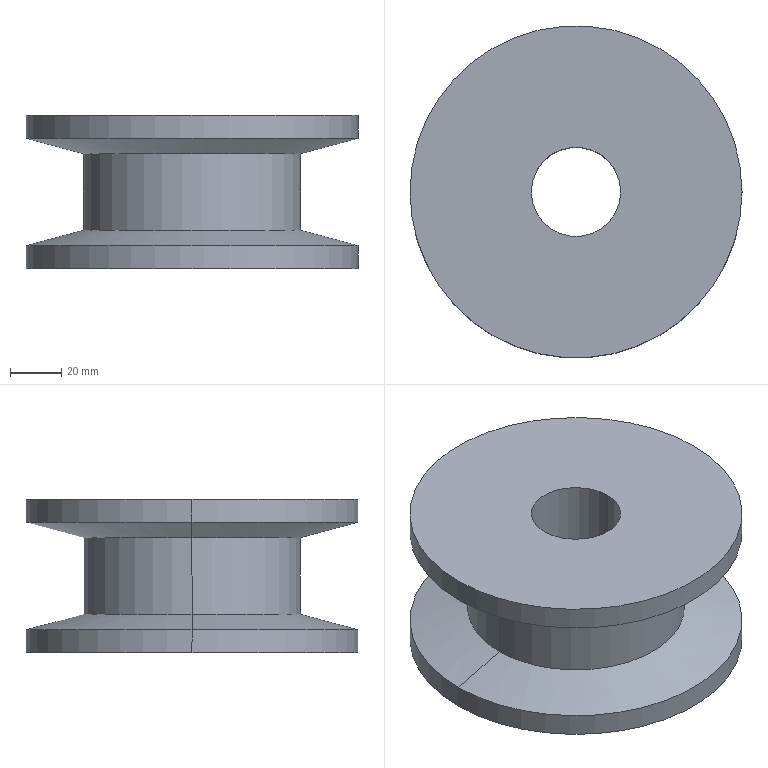Part | SolidWorks | features BaseBody 1 | 1 solid | 14 faces | box 130 x 130 x 60 mm | volume 461932 mm3 | cylinder 8 | cone 4 | plane 2 | commonest cylinder face diameters 130 x4 35 x2 85 x2
STEP:
#1=CARTESIAN_POINT('',(65.,0.,21.));
#2=VERTEX_POINT('',#1);
#3=CARTESIAN_POINT('',(-65.,0.,21.));
#4=VERTEX_POINT('',#3);
#5=CARTESIAN_POINT('',(0.,0.,21.));
#6=DIRECTION('',(0.,0.,1.));
#7=DIRECTION('',(1.,0.,0.));
#8=AXIS2_PLACEMENT_3D('',#5,#6,#7);
#9=CIRCLE('',#8,65.);
#10=EDGE_CURVE('',#2,#4,#9,.T.);
#11=ORIENTED_EDGE('',*,*,#10,.T.);
#12=CARTESIAN_POINT('',(-65.,0.,30.));
#13=VERTEX_POINT('',#12);
#14=CARTESIAN_POINT('',(-65.,0.,0.));
#15=DIRECTION('',(0.,0.,1.));
#16=VECTOR('',#15,1000.);
#17=LINE('',#14,#16);
#18=EDGE_CURVE('',#4,#13,#17,.T.);
#19=ORIENTED_EDGE('',*,*,#18,.T.);
#20=CARTESIAN_POINT('',(65.,0.,30.));
#21=VERTEX_POINT('',#20);
#22=CARTESIAN_POINT('',(0.,0.,30.));
#23=DIRECTION('',(0.,0.,-1.));
#24=DIRECTION('',(1.,0.,0.));
#25=AXIS2_PLACEMENT_3D('',#22,#23,#24);
#26=CIRCLE('',#25,65.);
#27=EDGE_CURVE('',#13,#21,#26,.T.);
#28=ORIENTED_EDGE('',*,*,#27,.T.);
#29=CARTESIAN_POINT('',(65.,0.,0.));
#30=DIRECTION('',(0.,0.,1.));
#31=VECTOR('',#30,1000.);
#32=LINE('',#29,#31);
#33=EDGE_CURVE('',#2,#21,#32,.T.);
#34=ORIENTED_EDGE('',*,*,#33,.F.);
#35=EDGE_LOOP('',(#11,#19,#28,#34));
#36=FACE_OUTER_BOUND('',#35,.T.);
#37=CARTESIAN_POINT('',(0.,0.,0.));
#38=DIRECTION('',(0.,0.,1.));
#39=DIRECTION('',(1.,0.,0.));
#40=AXIS2_PLACEMENT_3D('',#37,#38,#39);
#41=CYLINDRICAL_SURFACE('',#40,65.);
#42=ADVANCED_FACE('',(#36),#41,.T.);
#43=CARTESIAN_POINT('',(-17.5,0.,-30.));
#44=VERTEX_POINT('',#43);
#45=CARTESIAN_POINT('',(17.5,0.,-30.));
#46=VERTEX_POINT('',#45);
#47=CARTESIAN_POINT('',(0.,0.,-30.));
#48=DIRECTION('',(0.,0.,1.));
#49=DIRECTION('',(1.,0.,0.));
#50=AXIS2_PLACEMENT_3D('',#47,#48,#49);
#51=CIRCLE('',#50,17.5);
#52=EDGE_CURVE('',#44,#46,#51,.T.);
#53=ORIENTED_EDGE('',*,*,#52,.F.);
#54=CARTESIAN_POINT('',(-17.5,0.,30.));
#55=VERTEX_POINT('',#54);
#56=CARTESIAN_POINT('',(-17.5,0.,0.));
#57=DIRECTION('',(0.,0.,1.));
#58=VECTOR('',#57,1000.);
#59=LINE('',#56,#58);
#60=EDGE_CURVE('',#44,#55,#59,.T.);
#61=ORIENTED_EDGE('',*,*,#60,.T.);
#62=CARTESIAN_POINT('',(17.5,0.,30.));
#63=VERTEX_POINT('',#62);
#64=CARTESIAN_POINT('',(0.,0.,30.));
#65=DIRECTION('',(0.,0.,1.));
#66=DIRECTION('',(1.,0.,0.));
#67=AXIS2_PLACEMENT_3D('',#64,#65,#66);
#68=CIRCLE('',#67,17.5);
#69=EDGE_CURVE('',#55,#63,#68,.T.);
#70=ORIENTED_EDGE('',*,*,#69,.T.);
#71=CARTESIAN_POINT('',(17.5,0.,0.));
#72=DIRECTION('',(0.,0.,1.));
#73=VECTOR('',#72,1000.);
#74=LINE('',#71,#73);
#75=EDGE_CURVE('',#46,#63,#74,.T.);
#76=ORIENTED_EDGE('',*,*,#75,.F.);
#77=EDGE_LOOP('',(#53,#61,#70,#76));
#78=FACE_OUTER_BOUND('',#77,.T.);
#79=CARTESIAN_POINT('',(0.,0.,0.));
#80=DIRECTION('',(0.,0.,1.));
#81=DIRECTION('',(1.,0.,0.));
#82=AXIS2_PLACEMENT_3D('',#79,#80,#81);
#83=CYLINDRICAL_SURFACE('',#82,17.5);
#84=ADVANCED_FACE('',(#78),#83,.F.);
#85=CARTESIAN_POINT('',(42.5,0.,15.));
#86=VERTEX_POINT('',#85);
#87=CARTESIAN_POINT('',(-42.5,0.,15.));
#88=VERTEX_POINT('',#87);
#89=CARTESIAN_POINT('',(0.,0.,15.));
#90=DIRECTION('',(0.,0.,1.));
#91=DIRECTION('',(1.,0.,0.));
#92=AXIS2_PLACEMENT_3D('',#89,#90,#91);
#93=CIRCLE('',#92,42.5);
#94=EDGE_CURVE('',#86,#88,#93,.T.);
#95=ORIENTED_EDGE('',*,*,#94,.T.);
#96=CARTESIAN_POINT('',(-65.,0.,21.));
#97=DIRECTION('',(-0.9662,0.,0.2577));
#98=VECTOR('',#97,1000.);
#99=LINE('',#96,#98);
#100=EDGE_CURVE('',#88,#4,#99,.T.);
#101=ORIENTED_EDGE('',*,*,#100,.T.);
#102=ORIENTED_EDGE('',*,*,#10,.F.);
#103=CARTESIAN_POINT('',(65.,0.,21.));
#104=DIRECTION('',(0.9662,0.,0.2577));
#105=VECTOR('',#104,1000.);
#106=LINE('',#103,#105);
#107=EDGE_CURVE('',#86,#2,#106,.T.);
#108=ORIENTED_EDGE('',*,*,#107,.F.);
#109=EDGE_LOOP('',(#95,#101,#102,#108));
#110=FACE_OUTER_BOUND('',#109,.T.);
#111=CARTESIAN_POINT('',(0.,0.,21.));
#112=DIRECTION('',(0.,0.,1.));
#113=DIRECTION('',(1.,0.,0.));
#114=AXIS2_PLACEMENT_3D('',#111,#112,#113);
#115=CONICAL_SURFACE('',#114,65.,1.31);
#116=ADVANCED_FACE('',(#110),#115,.T.);
#117=CARTESIAN_POINT('',(42.5,0.,-15.));
#118=VERTEX_POINT('',#117);
#119=CARTESIAN_POINT('',(-42.5,0.,-15.));
#120=VERTEX_POINT('',#119);
#121=CARTESIAN_POINT('',(0.,0.,-15.));
#122=DIRECTION('',(0.,0.,1.));
#123=DIRECTION('',(1.,0.,0.));
#124=AXIS2_PLACEMENT_3D('',#121,#122,#123);
#125=CIRCLE('',#124,42.5);
#126=EDGE_CURVE('',#118,#120,#125,.T.);
#127=ORIENTED_EDGE('',*,*,#126,.T.);
#128=CARTESIAN_POINT('',(-42.5,0.,0.));
#129=DIRECTION('',(0.,0.,1.));
#130=VECTOR('',#129,1000.);
#131=LINE('',#128,#130);
#132=EDGE_CURVE('',#120,#88,#131,.T.);
#133=ORIENTED_EDGE('',*,*,#132,.T.);
#134=ORIENTED_EDGE('',*,*,#94,.F.);
#135=CARTESIAN_POINT('',(42.5,0.,0.));
#136=DIRECTION('',(0.,0.,1.));
#137=VECTOR('',#136,1000.);
#138=LINE('',#135,#137);
#139=EDGE_CURVE('',#118,#86,#138,.T.);
#140=ORIENTED_EDGE('',*,*,#139,.F.);
#141=EDGE_LOOP('',(#127,#133,#134,#140));
#142=FACE_OUTER_BOUND('',#141,.T.);
#143=CARTESIAN_POINT('',(0.,0.,0.));
#144=DIRECTION('',(0.,0.,1.));
#145=DIRECTION('',(1.,0.,0.));
#146=AXIS2_PLACEMENT_3D('',#143,#144,#145);
#147=CYLINDRICAL_SURFACE('',#146,42.5);
#148=ADVANCED_FACE('',(#142),#147,.T.);
#149=CARTESIAN_POINT('',(65.,0.,-30.));
#150=VERTEX_POINT('',#149);
#151=CARTESIAN_POINT('',(-65.,0.,-30.));
#152=VERTEX_POINT('',#151);
#153=CARTESIAN_POINT('',(0.,0.,-30.));
#154=DIRECTION('',(0.,0.,1.));
#155=DIRECTION('',(1.,0.,0.));
#156=AXIS2_PLACEMENT_3D('',#153,#154,#155);
#157=CIRCLE('',#156,65.);
#158=EDGE_CURVE('',#150,#152,#157,.T.);
#159=ORIENTED_EDGE('',*,*,#158,.T.);
#160=CARTESIAN_POINT('',(-65.,0.,-21.));
#161=VERTEX_POINT('',#160);
#162=CARTESIAN_POINT('',(-65.,0.,0.));
#163=DIRECTION('',(0.,0.,1.));
#164=VECTOR('',#163,1000.);
#165=LINE('',#162,#164);
#166=EDGE_CURVE('',#152,#161,#165,.T.);
#167=ORIENTED_EDGE('',*,*,#166,.T.);
#168=CARTESIAN_POINT('',(65.,0.,-21.));
#169=VERTEX_POINT('',#168);
#170=CARTESIAN_POINT('',(0.,0.,-21.));
#171=DIRECTION('',(0.,0.,-1.));
#172=DIRECTION('',(1.,0.,0.));
#173=AXIS2_PLACEMENT_3D('',#170,#171,#172);
#174=CIRCLE('',#173,65.);
#175=EDGE_CURVE('',#161,#169,#174,.T.);
#176=ORIENTED_EDGE('',*,*,#175,.T.);
#177=CARTESIAN_POINT('',(65.,0.,0.));
#178=DIRECTION('',(0.,0.,1.));
#179=VECTOR('',#178,1000.);
#180=LINE('',#177,#179);
#181=EDGE_CURVE('',#150,#169,#180,.T.);
#182=ORIENTED_EDGE('',*,*,#181,.F.);
#183=EDGE_LOOP('',(#159,#167,#176,#182));
#184=FACE_OUTER_BOUND('',#183,.T.);
#185=CARTESIAN_POINT('',(0.,0.,0.));
#186=DIRECTION('',(0.,0.,1.));
#187=DIRECTION('',(1.,0.,0.));
#188=AXIS2_PLACEMENT_3D('',#185,#186,#187);
#189=CYLINDRICAL_SURFACE('',#188,65.);
#190=ADVANCED_FACE('',(#184),#189,.T.);
#191=ORIENTED_EDGE('',*,*,#126,.F.);
#192=CARTESIAN_POINT('',(65.,0.,-21.));
#193=DIRECTION('',(0.9662,0.,-0.2577));
#194=VECTOR('',#193,1000.);
#195=LINE('',#192,#194);
#196=EDGE_CURVE('',#118,#169,#195,.T.);
#197=ORIENTED_EDGE('',*,*,#196,.T.);
#198=ORIENTED_EDGE('',*,*,#175,.F.);
#199=CARTESIAN_POINT('',(-65.,0.,-21.));
#200=DIRECTION('',(-0.9662,0.,-0.2577));
#201=VECTOR('',#200,1000.);
#202=LINE('',#199,#201);
#203=EDGE_CURVE('',#120,#161,#202,.T.);
#204=ORIENTED_EDGE('',*,*,#203,.F.);
#205=EDGE_LOOP('',(#191,#197,#198,#204));
#206=FACE_OUTER_BOUND('',#205,.T.);
#207=CARTESIAN_POINT('',(0.,0.,-21.));
#208=DIRECTION('',(0.,0.,-1.));
#209=DIRECTION('',(-1.,0.,0.));
#210=AXIS2_PLACEMENT_3D('',#207,#208,#209);
#211=CONICAL_SURFACE('',#210,65.,1.31);
#212=ADVANCED_FACE('',(#206),#211,.T.);
#213=CARTESIAN_POINT('',(0.,0.,30.));
#214=DIRECTION('',(0.,0.,-1.));
#215=DIRECTION('',(1.,0.,0.));
#216=AXIS2_PLACEMENT_3D('',#213,#214,#215);
#217=CIRCLE('',#216,65.);
#218=EDGE_CURVE('',#21,#13,#217,.T.);
#219=ORIENTED_EDGE('',*,*,#218,.F.);
#220=ORIENTED_EDGE('',*,*,#27,.F.);
#221=EDGE_LOOP('',(#219,#220));
#222=FACE_OUTER_BOUND('',#221,.T.);
#223=CARTESIAN_POINT('',(0.,0.,30.));
#224=DIRECTION('',(0.,0.,1.));
#225=DIRECTION('',(1.,0.,0.));
#226=AXIS2_PLACEMENT_3D('',#223,#224,#225);
#227=CIRCLE('',#226,17.5);
#228=EDGE_CURVE('',#63,#55,#227,.T.);
#229=ORIENTED_EDGE('',*,*,#228,.F.);
#230=ORIENTED_EDGE('',*,*,#69,.F.);
#231=EDGE_LOOP('',(#229,#230));
#232=FACE_BOUND('',#231,.T.);
#233=CARTESIAN_POINT('',(0.,17.5,30.));
#234=DIRECTION('',(0.,0.,-1.));
#235=DIRECTION('',(-1.,0.,0.));
#236=AXIS2_PLACEMENT_3D('',#233,#234,#235);
#237=PLANE('',#236);
#238=ADVANCED_FACE('',(#222,#232),#237,.F.);
#239=ORIENTED_EDGE('',*,*,#18,.F.);
#240=CARTESIAN_POINT('',(0.,0.,21.));
#241=DIRECTION('',(0.,0.,1.));
#242=DIRECTION('',(1.,0.,0.));
#243=AXIS2_PLACEMENT_3D('',#240,#241,#242);
#244=CIRCLE('',#243,65.);
#245=EDGE_CURVE('',#4,#2,#244,.T.);
#246=ORIENTED_EDGE('',*,*,#245,.T.);
#247=ORIENTED_EDGE('',*,*,#33,.T.);
#248=ORIENTED_EDGE('',*,*,#218,.T.);
#249=EDGE_LOOP('',(#239,#246,#247,#248));
#250=FACE_OUTER_BOUND('',#249,.T.);
#251=CARTESIAN_POINT('',(0.,0.,0.));
#252=DIRECTION('',(0.,0.,1.));
#253=DIRECTION('',(1.,0.,0.));
#254=AXIS2_PLACEMENT_3D('',#251,#252,#253);
#255=CYLINDRICAL_SURFACE('',#254,65.);
#256=ADVANCED_FACE('',(#250),#255,.T.);
#257=ORIENTED_EDGE('',*,*,#60,.F.);
#258=CARTESIAN_POINT('',(0.,0.,-30.));
#259=DIRECTION('',(0.,0.,1.));
#260=DIRECTION('',(1.,0.,0.));
#261=AXIS2_PLACEMENT_3D('',#258,#259,#260);
#262=CIRCLE('',#261,17.5);
#263=EDGE_CURVE('',#46,#44,#262,.T.);
#264=ORIENTED_EDGE('',*,*,#263,.F.);
#265=ORIENTED_EDGE('',*,*,#75,.T.);
#266=ORIENTED_EDGE('',*,*,#228,.T.);
#267=EDGE_LOOP('',(#257,#264,#265,#266));
#268=FACE_OUTER_BOUND('',#267,.T.);
#269=CARTESIAN_POINT('',(0.,0.,0.));
#270=DIRECTION('',(0.,0.,1.));
#271=DIRECTION('',(1.,0.,0.));
#272=AXIS2_PLACEMENT_3D('',#269,#270,#271);
#273=CYLINDRICAL_SURFACE('',#272,17.5);
#274=ADVANCED_FACE('',(#268),#273,.F.);
#275=ORIENTED_EDGE('',*,*,#100,.F.);
#276=CARTESIAN_POINT('',(0.,0.,15.));
#277=DIRECTION('',(0.,0.,1.));
#278=DIRECTION('',(1.,0.,0.));
#279=AXIS2_PLACEMENT_3D('',#276,#277,#278);
#280=CIRCLE('',#279,42.5);
#281=EDGE_CURVE('',#88,#86,#280,.T.);
#282=ORIENTED_EDGE('',*,*,#281,.T.);
#283=ORIENTED_EDGE('',*,*,#107,.T.);
#284=ORIENTED_EDGE('',*,*,#245,.F.);
#285=EDGE_LOOP('',(#275,#282,#283,#284));
#286=FACE_OUTER_BOUND('',#285,.T.);
#287=CARTESIAN_POINT('',(0.,0.,21.));
#288=DIRECTION('',(0.,0.,1.));
#289=DIRECTION('',(1.,0.,0.));
#290=AXIS2_PLACEMENT_3D('',#287,#288,#289);
#291=CONICAL_SURFACE('',#290,65.,1.31);
#292=ADVANCED_FACE('',(#286),#291,.T.);
#293=ORIENTED_EDGE('',*,*,#263,.T.);
#294=ORIENTED_EDGE('',*,*,#52,.T.);
#295=EDGE_LOOP('',(#293,#294));
#296=FACE_BOUND('',#295,.T.);
#297=ORIENTED_EDGE('',*,*,#158,.F.);
#298=CARTESIAN_POINT('',(0.,0.,-30.));
#299=DIRECTION('',(0.,0.,1.));
#300=DIRECTION('',(1.,0.,0.));
#301=AXIS2_PLACEMENT_3D('',#298,#299,#300);
#302=CIRCLE('',#301,65.);
#303=EDGE_CURVE('',#152,#150,#302,.T.);
#304=ORIENTED_EDGE('',*,*,#303,.F.);
#305=EDGE_LOOP('',(#297,#304));
#306=FACE_OUTER_BOUND('',#305,.T.);
#307=CARTESIAN_POINT('',(0.,17.5,-30.));
#308=DIRECTION('',(0.,0.,1.));
#309=DIRECTION('',(1.,0.,0.));
#310=AXIS2_PLACEMENT_3D('',#307,#308,#309);
#311=PLANE('',#310);
#312=ADVANCED_FACE('',(#296,#306),#311,.F.);
#313=ORIENTED_EDGE('',*,*,#132,.F.);
#314=CARTESIAN_POINT('',(0.,0.,-15.));
#315=DIRECTION('',(0.,0.,1.));
#316=DIRECTION('',(1.,0.,0.));
#317=AXIS2_PLACEMENT_3D('',#314,#315,#316);
#318=CIRCLE('',#317,42.5);
#319=EDGE_CURVE('',#120,#118,#318,.T.);
#320=ORIENTED_EDGE('',*,*,#319,.T.);
#321=ORIENTED_EDGE('',*,*,#139,.T.);
#322=ORIENTED_EDGE('',*,*,#281,.F.);
#323=EDGE_LOOP('',(#313,#320,#321,#322));
#324=FACE_OUTER_BOUND('',#323,.T.);
#325=CARTESIAN_POINT('',(0.,0.,0.));
#326=DIRECTION('',(0.,0.,1.));
#327=DIRECTION('',(1.,0.,0.));
#328=AXIS2_PLACEMENT_3D('',#325,#326,#327);
#329=CYLINDRICAL_SURFACE('',#328,42.5);
#330=ADVANCED_FACE('',(#324),#329,.T.);
#331=ORIENTED_EDGE('',*,*,#166,.F.);
#332=ORIENTED_EDGE('',*,*,#303,.T.);
#333=ORIENTED_EDGE('',*,*,#181,.T.);
#334=CARTESIAN_POINT('',(0.,0.,-21.));
#335=DIRECTION('',(0.,0.,-1.));
#336=DIRECTION('',(1.,0.,0.));
#337=AXIS2_PLACEMENT_3D('',#334,#335,#336);
#338=CIRCLE('',#337,65.);
#339=EDGE_CURVE('',#169,#161,#338,.T.);
#340=ORIENTED_EDGE('',*,*,#339,.T.);
#341=EDGE_LOOP('',(#331,#332,#333,#340));
#342=FACE_OUTER_BOUND('',#341,.T.);
#343=CARTESIAN_POINT('',(0.,0.,0.));
#344=DIRECTION('',(0.,0.,1.));
#345=DIRECTION('',(1.,0.,0.));
#346=AXIS2_PLACEMENT_3D('',#343,#344,#345);
#347=CYLINDRICAL_SURFACE('',#346,65.);
#348=ADVANCED_FACE('',(#342),#347,.T.);
#349=ORIENTED_EDGE('',*,*,#196,.F.);
#350=ORIENTED_EDGE('',*,*,#319,.F.);
#351=ORIENTED_EDGE('',*,*,#203,.T.);
#352=ORIENTED_EDGE('',*,*,#339,.F.);
#353=EDGE_LOOP('',(#349,#350,#351,#352));
#354=FACE_OUTER_BOUND('',#353,.T.);
#355=CARTESIAN_POINT('',(0.,0.,-21.));
#356=DIRECTION('',(0.,0.,-1.));
#357=DIRECTION('',(-1.,0.,0.));
#358=AXIS2_PLACEMENT_3D('',#355,#356,#357);
#359=CONICAL_SURFACE('',#358,65.,1.31);
#360=ADVANCED_FACE('',(#354),#359,.T.);
#361=CLOSED_SHELL('',(#42,#84,#116,#148,#190,#212,#238,#256,#274,#292,#312,#330,#348,#360));
#362=MANIFOLD_SOLID_BREP('',#361);
#363=CARTESIAN_POINT('',(0.,0.,0.));
#364=DIRECTION('',(0.,0.,1.));
#365=DIRECTION('',(1.,0.,0.));
#366=AXIS2_PLACEMENT_3D('',#363,#364,#365);
#367=(LENGTH_UNIT()NAMED_UNIT(*)SI_UNIT(.MILLI.,.METRE.));
#368=UNCERTAINTY_MEASURE_WITH_UNIT(LENGTH_MEASURE(0.00001),#367,'','');
#369=(NAMED_UNIT(*)PLANE_ANGLE_UNIT()SI_UNIT($,.RADIAN.));
#370=(NAMED_UNIT(*)SI_UNIT($,.STERADIAN.)SOLID_ANGLE_UNIT());
#371=(GEOMETRIC_REPRESENTATION_CONTEXT(3)GLOBAL_UNCERTAINTY_ASSIGNED_CONTEXT((#368))GLOBAL_UNIT_ASSIGNED_CONTEXT((#367,#369,#370))REPRESENTATION_CONTEXT('',''));
#372=ADVANCED_BREP_SHAPE_REPRESENTATION('',(#362,#366),#371);